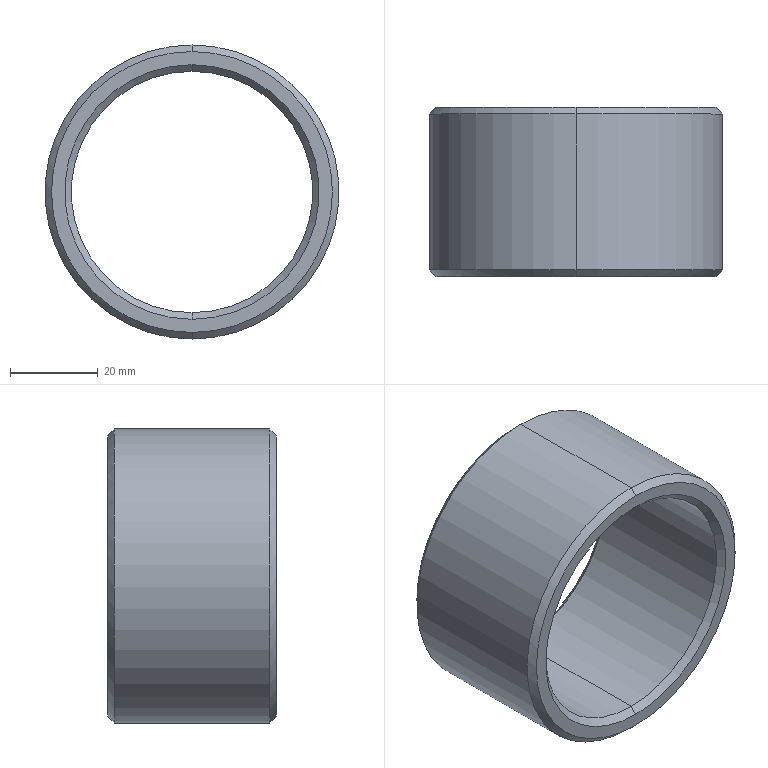Part | SolidWorks | features Chamfer 1, Extrusion 1 | 1 solid | 14 faces | box 67 x 38.5 x 67 mm | volume 43406 mm3 | cone 8 | cylinder 4 | plane 2 | commonest cylinder face diameters 55 x2 67 x2
STEP:
#1=CARTESIAN_POINT('',(0.,38.5,32.));
#2=VERTEX_POINT('',#1);
#3=CARTESIAN_POINT('',(0.,38.5,-32.));
#4=VERTEX_POINT('',#3);
#5=CARTESIAN_POINT('',(0.,38.5,0.));
#6=DIRECTION('',(0.,1.,0.));
#7=DIRECTION('',(0.,0.,1.));
#8=AXIS2_PLACEMENT_3D('',#5,#6,#7);
#9=CIRCLE('',#8,32.);
#10=EDGE_CURVE('',#2,#4,#9,.T.);
#11=ORIENTED_EDGE('',*,*,#10,.F.);
#12=CARTESIAN_POINT('',(0.,37.,33.5));
#13=VERTEX_POINT('',#12);
#14=CARTESIAN_POINT('',(0.,38.5,32.));
#15=DIRECTION('',(0.,-0.7071,0.7071));
#16=VECTOR('',#15,1000.);
#17=LINE('',#14,#16);
#18=EDGE_CURVE('',#2,#13,#17,.T.);
#19=ORIENTED_EDGE('',*,*,#18,.T.);
#20=CARTESIAN_POINT('',(0.,37.,-33.5));
#21=VERTEX_POINT('',#20);
#22=CARTESIAN_POINT('',(0.,37.,0.));
#23=DIRECTION('',(0.,-1.,0.));
#24=DIRECTION('',(0.,0.,1.));
#25=AXIS2_PLACEMENT_3D('',#22,#23,#24);
#26=CIRCLE('',#25,33.5);
#27=EDGE_CURVE('',#21,#13,#26,.T.);
#28=ORIENTED_EDGE('',*,*,#27,.F.);
#29=CARTESIAN_POINT('',(0.,38.5,-32.));
#30=DIRECTION('',(0.,-0.7071,-0.7071));
#31=VECTOR('',#30,1000.);
#32=LINE('',#29,#31);
#33=EDGE_CURVE('',#4,#21,#32,.T.);
#34=ORIENTED_EDGE('',*,*,#33,.F.);
#35=EDGE_LOOP('',(#11,#19,#28,#34));
#36=FACE_OUTER_BOUND('',#35,.T.);
#37=CARTESIAN_POINT('',(0.,38.5,0.));
#38=DIRECTION('',(0.,-1.,0.));
#39=DIRECTION('',(0.,0.,-1.));
#40=AXIS2_PLACEMENT_3D('',#37,#38,#39);
#41=CONICAL_SURFACE('',#40,32.,0.7854);
#42=ADVANCED_FACE('',(#36),#41,.T.);
#43=CARTESIAN_POINT('',(0.,37.,-27.5));
#44=VERTEX_POINT('',#43);
#45=CARTESIAN_POINT('',(0.,37.,27.5));
#46=VERTEX_POINT('',#45);
#47=CARTESIAN_POINT('',(0.,37.,0.));
#48=DIRECTION('',(0.,1.,0.));
#49=DIRECTION('',(0.,0.,1.));
#50=AXIS2_PLACEMENT_3D('',#47,#48,#49);
#51=CIRCLE('',#50,27.5);
#52=EDGE_CURVE('',#44,#46,#51,.T.);
#53=ORIENTED_EDGE('',*,*,#52,.F.);
#54=CARTESIAN_POINT('',(0.,38.5,-29.));
#55=VERTEX_POINT('',#54);
#56=CARTESIAN_POINT('',(0.,37.,-27.5));
#57=DIRECTION('',(0.,0.7071,-0.7071));
#58=VECTOR('',#57,1000.);
#59=LINE('',#56,#58);
#60=EDGE_CURVE('',#44,#55,#59,.T.);
#61=ORIENTED_EDGE('',*,*,#60,.T.);
#62=CARTESIAN_POINT('',(0.,38.5,29.));
#63=VERTEX_POINT('',#62);
#64=CARTESIAN_POINT('',(0.,38.5,0.));
#65=DIRECTION('',(0.,-1.,0.));
#66=DIRECTION('',(0.,0.,1.));
#67=AXIS2_PLACEMENT_3D('',#64,#65,#66);
#68=CIRCLE('',#67,29.);
#69=EDGE_CURVE('',#63,#55,#68,.T.);
#70=ORIENTED_EDGE('',*,*,#69,.F.);
#71=CARTESIAN_POINT('',(0.,37.,27.5));
#72=DIRECTION('',(0.,0.7071,0.7071));
#73=VECTOR('',#72,1000.);
#74=LINE('',#71,#73);
#75=EDGE_CURVE('',#46,#63,#74,.T.);
#76=ORIENTED_EDGE('',*,*,#75,.F.);
#77=EDGE_LOOP('',(#53,#61,#70,#76));
#78=FACE_OUTER_BOUND('',#77,.T.);
#79=CARTESIAN_POINT('',(0.,37.,0.));
#80=DIRECTION('',(0.,1.,0.));
#81=DIRECTION('',(0.,0.,1.));
#82=AXIS2_PLACEMENT_3D('',#79,#80,#81);
#83=CONICAL_SURFACE('',#82,27.5,0.7854);
#84=ADVANCED_FACE('',(#78),#83,.F.);
#85=CARTESIAN_POINT('',(0.,0.,-32.));
#86=VERTEX_POINT('',#85);
#87=CARTESIAN_POINT('',(0.,0.,32.));
#88=VERTEX_POINT('',#87);
#89=CARTESIAN_POINT('',(0.,0.,0.));
#90=DIRECTION('',(0.,-1.,0.));
#91=DIRECTION('',(0.,0.,1.));
#92=AXIS2_PLACEMENT_3D('',#89,#90,#91);
#93=CIRCLE('',#92,32.);
#94=EDGE_CURVE('',#86,#88,#93,.T.);
#95=ORIENTED_EDGE('',*,*,#94,.F.);
#96=CARTESIAN_POINT('',(0.,1.5,-33.5));
#97=VERTEX_POINT('',#96);
#98=CARTESIAN_POINT('',(0.,1.5,-33.5));
#99=DIRECTION('',(0.,0.7071,-0.7071));
#100=VECTOR('',#99,1000.);
#101=LINE('',#98,#100);
#102=EDGE_CURVE('',#86,#97,#101,.T.);
#103=ORIENTED_EDGE('',*,*,#102,.T.);
#104=CARTESIAN_POINT('',(0.,1.5,33.5));
#105=VERTEX_POINT('',#104);
#106=CARTESIAN_POINT('',(0.,1.5,0.));
#107=DIRECTION('',(0.,1.,0.));
#108=DIRECTION('',(0.,0.,1.));
#109=AXIS2_PLACEMENT_3D('',#106,#107,#108);
#110=CIRCLE('',#109,33.5);
#111=EDGE_CURVE('',#105,#97,#110,.T.);
#112=ORIENTED_EDGE('',*,*,#111,.F.);
#113=CARTESIAN_POINT('',(0.,1.5,33.5));
#114=DIRECTION('',(0.,0.7071,0.7071));
#115=VECTOR('',#114,1000.);
#116=LINE('',#113,#115);
#117=EDGE_CURVE('',#88,#105,#116,.T.);
#118=ORIENTED_EDGE('',*,*,#117,.F.);
#119=EDGE_LOOP('',(#95,#103,#112,#118));
#120=FACE_OUTER_BOUND('',#119,.T.);
#121=CARTESIAN_POINT('',(0.,1.5,0.));
#122=DIRECTION('',(0.,1.,0.));
#123=DIRECTION('',(0.,0.,1.));
#124=AXIS2_PLACEMENT_3D('',#121,#122,#123);
#125=CONICAL_SURFACE('',#124,33.5,0.7854);
#126=ADVANCED_FACE('',(#120),#125,.T.);
#127=CARTESIAN_POINT('',(0.,1.5,27.5));
#128=VERTEX_POINT('',#127);
#129=CARTESIAN_POINT('',(0.,1.5,-27.5));
#130=VERTEX_POINT('',#129);
#131=CARTESIAN_POINT('',(0.,1.5,0.));
#132=DIRECTION('',(0.,-1.,0.));
#133=DIRECTION('',(0.,0.,1.));
#134=AXIS2_PLACEMENT_3D('',#131,#132,#133);
#135=CIRCLE('',#134,27.5);
#136=EDGE_CURVE('',#128,#130,#135,.T.);
#137=ORIENTED_EDGE('',*,*,#136,.F.);
#138=CARTESIAN_POINT('',(0.,0.,29.));
#139=VERTEX_POINT('',#138);
#140=CARTESIAN_POINT('',(0.,0.,29.));
#141=DIRECTION('',(0.,-0.7071,0.7071));
#142=VECTOR('',#141,1000.);
#143=LINE('',#140,#142);
#144=EDGE_CURVE('',#128,#139,#143,.T.);
#145=ORIENTED_EDGE('',*,*,#144,.T.);
#146=CARTESIAN_POINT('',(0.,0.,-29.));
#147=VERTEX_POINT('',#146);
#148=CARTESIAN_POINT('',(0.,0.,0.));
#149=DIRECTION('',(0.,1.,0.));
#150=DIRECTION('',(0.,0.,1.));
#151=AXIS2_PLACEMENT_3D('',#148,#149,#150);
#152=CIRCLE('',#151,29.);
#153=EDGE_CURVE('',#147,#139,#152,.T.);
#154=ORIENTED_EDGE('',*,*,#153,.F.);
#155=CARTESIAN_POINT('',(0.,0.,-29.));
#156=DIRECTION('',(0.,-0.7071,-0.7071));
#157=VECTOR('',#156,1000.);
#158=LINE('',#155,#157);
#159=EDGE_CURVE('',#130,#147,#158,.T.);
#160=ORIENTED_EDGE('',*,*,#159,.F.);
#161=EDGE_LOOP('',(#137,#145,#154,#160));
#162=FACE_OUTER_BOUND('',#161,.T.);
#163=CARTESIAN_POINT('',(0.,0.,0.));
#164=DIRECTION('',(0.,-1.,0.));
#165=DIRECTION('',(0.,0.,-1.));
#166=AXIS2_PLACEMENT_3D('',#163,#164,#165);
#167=CONICAL_SURFACE('',#166,29.,0.7854);
#168=ADVANCED_FACE('',(#162),#167,.F.);
#169=ORIENTED_EDGE('',*,*,#52,.T.);
#170=CARTESIAN_POINT('',(0.,38.5,27.5));
#171=DIRECTION('',(0.,-1.,0.));
#172=VECTOR('',#171,1000.);
#173=LINE('',#170,#172);
#174=EDGE_CURVE('',#46,#128,#173,.T.);
#175=ORIENTED_EDGE('',*,*,#174,.T.);
#176=ORIENTED_EDGE('',*,*,#136,.T.);
#177=CARTESIAN_POINT('',(0.,38.5,-27.5));
#178=DIRECTION('',(0.,-1.,0.));
#179=VECTOR('',#178,1000.);
#180=LINE('',#177,#179);
#181=EDGE_CURVE('',#44,#130,#180,.T.);
#182=ORIENTED_EDGE('',*,*,#181,.F.);
#183=EDGE_LOOP('',(#169,#175,#176,#182));
#184=FACE_OUTER_BOUND('',#183,.T.);
#185=CARTESIAN_POINT('',(0.,38.5,0.));
#186=DIRECTION('',(0.,-1.,0.));
#187=DIRECTION('',(0.,0.,-1.));
#188=AXIS2_PLACEMENT_3D('',#185,#186,#187);
#189=CYLINDRICAL_SURFACE('',#188,27.5);
#190=ADVANCED_FACE('',(#184),#189,.F.);
#191=ORIENTED_EDGE('',*,*,#27,.T.);
#192=CARTESIAN_POINT('',(0.,38.5,33.5));
#193=DIRECTION('',(0.,-1.,0.));
#194=VECTOR('',#193,1000.);
#195=LINE('',#192,#194);
#196=EDGE_CURVE('',#13,#105,#195,.T.);
#197=ORIENTED_EDGE('',*,*,#196,.T.);
#198=ORIENTED_EDGE('',*,*,#111,.T.);
#199=CARTESIAN_POINT('',(0.,38.5,-33.5));
#200=DIRECTION('',(0.,-1.,0.));
#201=VECTOR('',#200,1000.);
#202=LINE('',#199,#201);
#203=EDGE_CURVE('',#21,#97,#202,.T.);
#204=ORIENTED_EDGE('',*,*,#203,.F.);
#205=EDGE_LOOP('',(#191,#197,#198,#204));
#206=FACE_OUTER_BOUND('',#205,.T.);
#207=CARTESIAN_POINT('',(0.,38.5,0.));
#208=DIRECTION('',(0.,-1.,0.));
#209=DIRECTION('',(0.,0.,-1.));
#210=AXIS2_PLACEMENT_3D('',#207,#208,#209);
#211=CYLINDRICAL_SURFACE('',#210,33.5);
#212=ADVANCED_FACE('',(#206),#211,.T.);
#213=ORIENTED_EDGE('',*,*,#69,.T.);
#214=CARTESIAN_POINT('',(0.,38.5,0.));
#215=DIRECTION('',(0.,-1.,0.));
#216=DIRECTION('',(0.,0.,1.));
#217=AXIS2_PLACEMENT_3D('',#214,#215,#216);
#218=CIRCLE('',#217,29.);
#219=EDGE_CURVE('',#55,#63,#218,.T.);
#220=ORIENTED_EDGE('',*,*,#219,.T.);
#221=EDGE_LOOP('',(#213,#220));
#222=FACE_BOUND('',#221,.T.);
#223=CARTESIAN_POINT('',(0.,38.5,0.));
#224=DIRECTION('',(0.,1.,0.));
#225=DIRECTION('',(0.,0.,1.));
#226=AXIS2_PLACEMENT_3D('',#223,#224,#225);
#227=CIRCLE('',#226,32.);
#228=EDGE_CURVE('',#4,#2,#227,.T.);
#229=ORIENTED_EDGE('',*,*,#228,.T.);
#230=ORIENTED_EDGE('',*,*,#10,.T.);
#231=EDGE_LOOP('',(#229,#230));
#232=FACE_OUTER_BOUND('',#231,.T.);
#233=CARTESIAN_POINT('',(0.,38.5,0.));
#234=DIRECTION('',(0.,1.,0.));
#235=DIRECTION('',(0.,0.,1.));
#236=AXIS2_PLACEMENT_3D('',#233,#234,#235);
#237=PLANE('',#236);
#238=ADVANCED_FACE('',(#222,#232),#237,.T.);
#239=ORIENTED_EDGE('',*,*,#153,.T.);
#240=CARTESIAN_POINT('',(0.,0.,0.));
#241=DIRECTION('',(0.,1.,0.));
#242=DIRECTION('',(0.,0.,1.));
#243=AXIS2_PLACEMENT_3D('',#240,#241,#242);
#244=CIRCLE('',#243,29.);
#245=EDGE_CURVE('',#139,#147,#244,.T.);
#246=ORIENTED_EDGE('',*,*,#245,.T.);
#247=EDGE_LOOP('',(#239,#246));
#248=FACE_BOUND('',#247,.T.);
#249=CARTESIAN_POINT('',(0.,0.,0.));
#250=DIRECTION('',(0.,-1.,0.));
#251=DIRECTION('',(0.,0.,1.));
#252=AXIS2_PLACEMENT_3D('',#249,#250,#251);
#253=CIRCLE('',#252,32.);
#254=EDGE_CURVE('',#88,#86,#253,.T.);
#255=ORIENTED_EDGE('',*,*,#254,.T.);
#256=ORIENTED_EDGE('',*,*,#94,.T.);
#257=EDGE_LOOP('',(#255,#256));
#258=FACE_OUTER_BOUND('',#257,.T.);
#259=CARTESIAN_POINT('',(0.,0.,0.));
#260=DIRECTION('',(0.,1.,0.));
#261=DIRECTION('',(0.,0.,1.));
#262=AXIS2_PLACEMENT_3D('',#259,#260,#261);
#263=PLANE('',#262);
#264=ADVANCED_FACE('',(#248,#258),#263,.F.);
#265=ORIENTED_EDGE('',*,*,#196,.F.);
#266=CARTESIAN_POINT('',(0.,37.,0.));
#267=DIRECTION('',(0.,-1.,0.));
#268=DIRECTION('',(0.,0.,1.));
#269=AXIS2_PLACEMENT_3D('',#266,#267,#268);
#270=CIRCLE('',#269,33.5);
#271=EDGE_CURVE('',#13,#21,#270,.T.);
#272=ORIENTED_EDGE('',*,*,#271,.T.);
#273=ORIENTED_EDGE('',*,*,#203,.T.);
#274=CARTESIAN_POINT('',(0.,1.5,0.));
#275=DIRECTION('',(0.,1.,0.));
#276=DIRECTION('',(0.,0.,1.));
#277=AXIS2_PLACEMENT_3D('',#274,#275,#276);
#278=CIRCLE('',#277,33.5);
#279=EDGE_CURVE('',#97,#105,#278,.T.);
#280=ORIENTED_EDGE('',*,*,#279,.T.);
#281=EDGE_LOOP('',(#265,#272,#273,#280));
#282=FACE_OUTER_BOUND('',#281,.T.);
#283=CARTESIAN_POINT('',(0.,38.5,0.));
#284=DIRECTION('',(0.,-1.,0.));
#285=DIRECTION('',(0.,0.,-1.));
#286=AXIS2_PLACEMENT_3D('',#283,#284,#285);
#287=CYLINDRICAL_SURFACE('',#286,33.5);
#288=ADVANCED_FACE('',(#282),#287,.T.);
#289=ORIENTED_EDGE('',*,*,#174,.F.);
#290=CARTESIAN_POINT('',(0.,37.,0.));
#291=DIRECTION('',(0.,1.,0.));
#292=DIRECTION('',(0.,0.,1.));
#293=AXIS2_PLACEMENT_3D('',#290,#291,#292);
#294=CIRCLE('',#293,27.5);
#295=EDGE_CURVE('',#46,#44,#294,.T.);
#296=ORIENTED_EDGE('',*,*,#295,.T.);
#297=ORIENTED_EDGE('',*,*,#181,.T.);
#298=CARTESIAN_POINT('',(0.,1.5,0.));
#299=DIRECTION('',(0.,-1.,0.));
#300=DIRECTION('',(0.,0.,1.));
#301=AXIS2_PLACEMENT_3D('',#298,#299,#300);
#302=CIRCLE('',#301,27.5);
#303=EDGE_CURVE('',#130,#128,#302,.T.);
#304=ORIENTED_EDGE('',*,*,#303,.T.);
#305=EDGE_LOOP('',(#289,#296,#297,#304));
#306=FACE_OUTER_BOUND('',#305,.T.);
#307=CARTESIAN_POINT('',(0.,38.5,0.));
#308=DIRECTION('',(0.,-1.,0.));
#309=DIRECTION('',(0.,0.,-1.));
#310=AXIS2_PLACEMENT_3D('',#307,#308,#309);
#311=CYLINDRICAL_SURFACE('',#310,27.5);
#312=ADVANCED_FACE('',(#306),#311,.F.);
#313=ORIENTED_EDGE('',*,*,#144,.F.);
#314=ORIENTED_EDGE('',*,*,#303,.F.);
#315=ORIENTED_EDGE('',*,*,#159,.T.);
#316=ORIENTED_EDGE('',*,*,#245,.F.);
#317=EDGE_LOOP('',(#313,#314,#315,#316));
#318=FACE_OUTER_BOUND('',#317,.T.);
#319=CARTESIAN_POINT('',(0.,0.,0.));
#320=DIRECTION('',(0.,-1.,0.));
#321=DIRECTION('',(0.,0.,-1.));
#322=AXIS2_PLACEMENT_3D('',#319,#320,#321);
#323=CONICAL_SURFACE('',#322,29.,0.7854);
#324=ADVANCED_FACE('',(#318),#323,.F.);
#325=ORIENTED_EDGE('',*,*,#102,.F.);
#326=ORIENTED_EDGE('',*,*,#254,.F.);
#327=ORIENTED_EDGE('',*,*,#117,.T.);
#328=ORIENTED_EDGE('',*,*,#279,.F.);
#329=EDGE_LOOP('',(#325,#326,#327,#328));
#330=FACE_OUTER_BOUND('',#329,.T.);
#331=CARTESIAN_POINT('',(0.,1.5,0.));
#332=DIRECTION('',(0.,1.,0.));
#333=DIRECTION('',(0.,0.,1.));
#334=AXIS2_PLACEMENT_3D('',#331,#332,#333);
#335=CONICAL_SURFACE('',#334,33.5,0.7854);
#336=ADVANCED_FACE('',(#330),#335,.T.);
#337=ORIENTED_EDGE('',*,*,#60,.F.);
#338=ORIENTED_EDGE('',*,*,#295,.F.);
#339=ORIENTED_EDGE('',*,*,#75,.T.);
#340=ORIENTED_EDGE('',*,*,#219,.F.);
#341=EDGE_LOOP('',(#337,#338,#339,#340));
#342=FACE_OUTER_BOUND('',#341,.T.);
#343=CARTESIAN_POINT('',(0.,37.,0.));
#344=DIRECTION('',(0.,1.,0.));
#345=DIRECTION('',(0.,0.,1.));
#346=AXIS2_PLACEMENT_3D('',#343,#344,#345);
#347=CONICAL_SURFACE('',#346,27.5,0.7854);
#348=ADVANCED_FACE('',(#342),#347,.F.);
#349=ORIENTED_EDGE('',*,*,#18,.F.);
#350=ORIENTED_EDGE('',*,*,#228,.F.);
#351=ORIENTED_EDGE('',*,*,#33,.T.);
#352=ORIENTED_EDGE('',*,*,#271,.F.);
#353=EDGE_LOOP('',(#349,#350,#351,#352));
#354=FACE_OUTER_BOUND('',#353,.T.);
#355=CARTESIAN_POINT('',(0.,38.5,0.));
#356=DIRECTION('',(0.,-1.,0.));
#357=DIRECTION('',(0.,0.,-1.));
#358=AXIS2_PLACEMENT_3D('',#355,#356,#357);
#359=CONICAL_SURFACE('',#358,32.,0.7854);
#360=ADVANCED_FACE('',(#354),#359,.T.);
#361=CLOSED_SHELL('',(#42,#84,#126,#168,#190,#212,#238,#264,#288,#312,#324,#336,#348,#360));
#362=MANIFOLD_SOLID_BREP('',#361);
#363=CARTESIAN_POINT('',(0.,0.,0.));
#364=DIRECTION('',(0.,0.,1.));
#365=DIRECTION('',(1.,0.,0.));
#366=AXIS2_PLACEMENT_3D('',#363,#364,#365);
#367=(LENGTH_UNIT()NAMED_UNIT(*)SI_UNIT(.MILLI.,.METRE.));
#368=UNCERTAINTY_MEASURE_WITH_UNIT(LENGTH_MEASURE(0.00001),#367,'','');
#369=(NAMED_UNIT(*)PLANE_ANGLE_UNIT()SI_UNIT($,.RADIAN.));
#370=(NAMED_UNIT(*)SI_UNIT($,.STERADIAN.)SOLID_ANGLE_UNIT());
#371=(GEOMETRIC_REPRESENTATION_CONTEXT(3)GLOBAL_UNCERTAINTY_ASSIGNED_CONTEXT((#368))GLOBAL_UNIT_ASSIGNED_CONTEXT((#367,#369,#370))REPRESENTATION_CONTEXT('',''));
#372=ADVANCED_BREP_SHAPE_REPRESENTATION('',(#362,#366),#371);